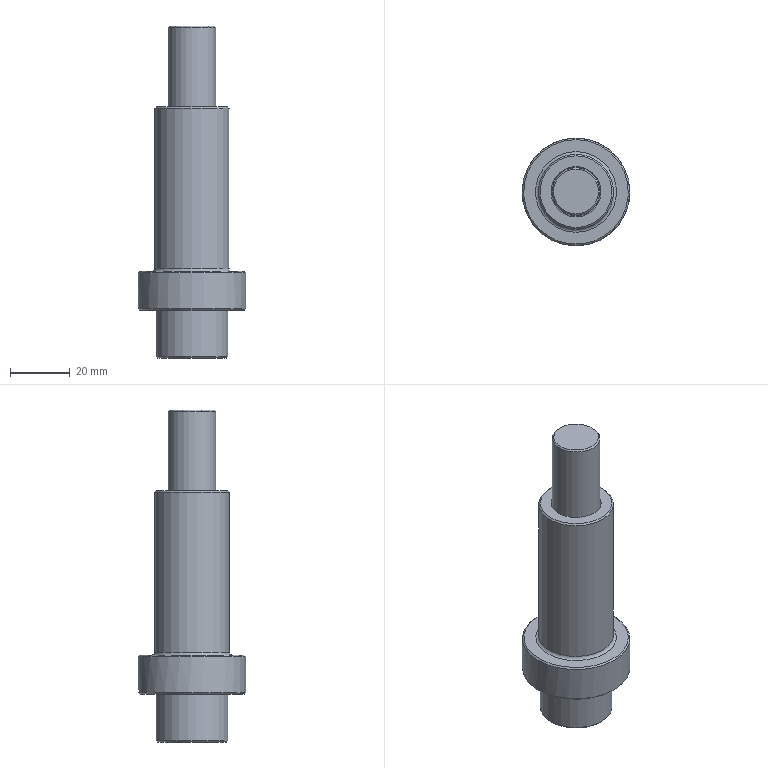Part | NX | features solid 2 | 1 solid | 97 faces | box 36 x 36 x 111 mm | volume 49252 mm3 | plane 56 | spline 30 | cylinder 5 | cone 5 | torus 1 | commonest cylinder face diameters 16 x1 16.8 x1 24 x1 25 x1 36 x1